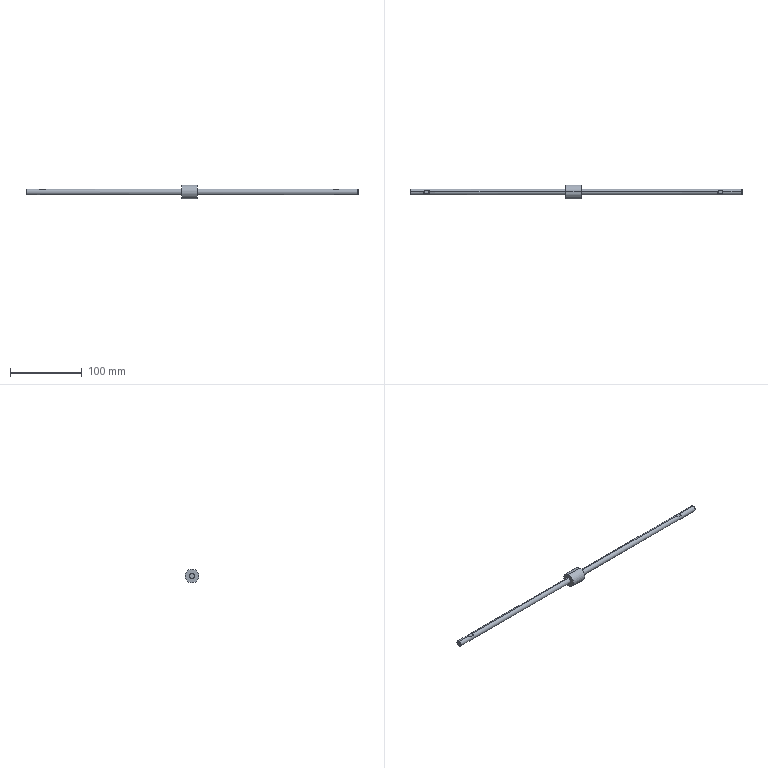Part | STEP file | _20MACJ15010Rod | 1 solid | 26 faces | box 463 x 19.5 x 19.5 mm | volume 28625 mm3 | plane 16 | cylinder 6 | cone 4 | commonest cylinder face diameters 8 x4 19.5 x2
STEP:
#1=CARTESIAN_POINT('',(462.233,0.,4.));
#2=VERTEX_POINT('',#1);
#3=CARTESIAN_POINT('',(462.233,0.,-4.));
#4=VERTEX_POINT('',#3);
#5=CARTESIAN_POINT('',(462.233,0.,0.));
#6=DIRECTION('',(-1.,0.,0.));
#7=DIRECTION('',(0.,0.,1.));
#8=AXIS2_PLACEMENT_3D('',#5,#6,#7);
#9=CIRCLE('',#8,4.);
#10=EDGE_CURVE('',#2,#4,#9,.T.);
#11=ORIENTED_EDGE('',*,*,#10,.T.);
#12=CARTESIAN_POINT('',(436.,0.,-4.));
#13=VERTEX_POINT('',#12);
#14=CARTESIAN_POINT('',(463.,0.,-4.));
#15=DIRECTION('',(-1.,0.,0.));
#16=VECTOR('',#15,1000.);
#17=LINE('',#14,#16);
#18=EDGE_CURVE('',#4,#13,#17,.T.);
#19=ORIENTED_EDGE('',*,*,#18,.T.);
#20=CARTESIAN_POINT('',(436.,2.646,-3.));
#21=VERTEX_POINT('',#20);
#22=CARTESIAN_POINT('',(436.,0.,0.));
#23=DIRECTION('',(1.,0.,0.));
#24=DIRECTION('',(0.,0.,1.));
#25=AXIS2_PLACEMENT_3D('',#22,#23,#24);
#26=CIRCLE('',#25,4.);
#27=EDGE_CURVE('',#13,#21,#26,.T.);
#28=ORIENTED_EDGE('',*,*,#27,.T.);
#29=CARTESIAN_POINT('',(430.,2.646,-3.));
#30=VERTEX_POINT('',#29);
#31=CARTESIAN_POINT('',(463.,2.646,-3.));
#32=DIRECTION('',(-1.,0.,0.));
#33=VECTOR('',#32,1000.);
#34=LINE('',#31,#33);
#35=EDGE_CURVE('',#21,#30,#34,.T.);
#36=ORIENTED_EDGE('',*,*,#35,.T.);
#37=CARTESIAN_POINT('',(429.,0.,-4.));
#38=VERTEX_POINT('',#37);
#39=CARTESIAN_POINT('',(430.,2.646,-3.));
#40=CARTESIAN_POINT('',(429.348,1.907,-3.652));
#41=CARTESIAN_POINT('',(429.,0.9852,-4.));
#42=CARTESIAN_POINT('',(429.,0.,-4.));
#43=(BOUNDED_CURVE()B_SPLINE_CURVE(3,(#39,#40,#41,#42),.UNSPECIFIED.,.F.,.T.)B_SPLINE_CURVE_WITH_KNOTS((4,4),(5.56,6.283),.UNSPECIFIED.)CURVE()GEOMETRIC_REPRESENTATION_ITEM()RATIONAL_B_SPLINE_CURVE((1.,0.9569,0.9569,1.))REPRESENTATION_ITEM(''));
#44=EDGE_CURVE('',#30,#38,#43,.T.);
#45=ORIENTED_EDGE('',*,*,#44,.T.);
#46=CARTESIAN_POINT('',(239.,0.,-4.));
#47=VERTEX_POINT('',#46);
#48=CARTESIAN_POINT('',(463.,0.,-4.));
#49=DIRECTION('',(-1.,0.,0.));
#50=VECTOR('',#49,1000.);
#51=LINE('',#48,#50);
#52=EDGE_CURVE('',#38,#47,#51,.T.);
#53=ORIENTED_EDGE('',*,*,#52,.T.);
#54=CARTESIAN_POINT('',(239.,0.,4.));
#55=VERTEX_POINT('',#54);
#56=CARTESIAN_POINT('',(239.,0.,0.));
#57=DIRECTION('',(1.,0.,0.));
#58=DIRECTION('',(0.,0.,1.));
#59=AXIS2_PLACEMENT_3D('',#56,#57,#58);
#60=CIRCLE('',#59,4.);
#61=EDGE_CURVE('',#47,#55,#60,.T.);
#62=ORIENTED_EDGE('',*,*,#61,.T.);
#63=CARTESIAN_POINT('',(429.,0.,4.));
#64=VERTEX_POINT('',#63);
#65=CARTESIAN_POINT('',(463.,0.,4.));
#66=DIRECTION('',(-1.,0.,0.));
#67=VECTOR('',#66,1000.);
#68=LINE('',#65,#67);
#69=EDGE_CURVE('',#64,#55,#68,.T.);
#70=ORIENTED_EDGE('',*,*,#69,.F.);
#71=CARTESIAN_POINT('',(430.,2.646,3.));
#72=VERTEX_POINT('',#71);
#73=CARTESIAN_POINT('',(429.,0.,4.));
#74=CARTESIAN_POINT('',(429.,0.9852,4.));
#75=CARTESIAN_POINT('',(429.348,1.907,3.652));
#76=CARTESIAN_POINT('',(430.,2.646,3.));
#77=(BOUNDED_CURVE()B_SPLINE_CURVE(3,(#73,#74,#75,#76),.UNSPECIFIED.,.F.,.T.)B_SPLINE_CURVE_WITH_KNOTS((4,4),(0.,0.7227),.UNSPECIFIED.)CURVE()GEOMETRIC_REPRESENTATION_ITEM()RATIONAL_B_SPLINE_CURVE((1.,0.9569,0.9569,1.))REPRESENTATION_ITEM(''));
#78=EDGE_CURVE('',#64,#72,#77,.T.);
#79=ORIENTED_EDGE('',*,*,#78,.T.);
#80=CARTESIAN_POINT('',(436.,2.646,3.));
#81=VERTEX_POINT('',#80);
#82=CARTESIAN_POINT('',(463.,2.646,3.));
#83=DIRECTION('',(1.,0.,0.));
#84=VECTOR('',#83,1000.);
#85=LINE('',#82,#84);
#86=EDGE_CURVE('',#72,#81,#85,.T.);
#87=ORIENTED_EDGE('',*,*,#86,.T.);
#88=CARTESIAN_POINT('',(436.,0.,4.));
#89=VERTEX_POINT('',#88);
#90=CARTESIAN_POINT('',(436.,0.,0.));
#91=DIRECTION('',(1.,0.,0.));
#92=DIRECTION('',(0.,0.,1.));
#93=AXIS2_PLACEMENT_3D('',#90,#91,#92);
#94=CIRCLE('',#93,4.);
#95=EDGE_CURVE('',#81,#89,#94,.T.);
#96=ORIENTED_EDGE('',*,*,#95,.T.);
#97=CARTESIAN_POINT('',(463.,0.,4.));
#98=DIRECTION('',(-1.,0.,0.));
#99=VECTOR('',#98,1000.);
#100=LINE('',#97,#99);
#101=EDGE_CURVE('',#2,#89,#100,.T.);
#102=ORIENTED_EDGE('',*,*,#101,.F.);
#103=EDGE_LOOP('',(#11,#19,#28,#36,#45,#53,#62,#70,#79,#87,#96,#102));
#104=FACE_OUTER_BOUND('',#103,.T.);
#105=CARTESIAN_POINT('',(463.,0.,0.));
#106=DIRECTION('',(-1.,0.,0.));
#107=DIRECTION('',(0.,0.,1.));
#108=AXIS2_PLACEMENT_3D('',#105,#106,#107);
#109=CYLINDRICAL_SURFACE('',#108,4.);
#110=ADVANCED_FACE('',(#104),#109,.T.);
#111=CARTESIAN_POINT('',(463.,0.,3.233));
#112=VERTEX_POINT('',#111);
#113=CARTESIAN_POINT('',(463.,0.,-3.233));
#114=VERTEX_POINT('',#113);
#115=CARTESIAN_POINT('',(463.,0.,0.));
#116=DIRECTION('',(-1.,0.,0.));
#117=DIRECTION('',(0.,0.,1.));
#118=AXIS2_PLACEMENT_3D('',#115,#116,#117);
#119=CIRCLE('',#118,3.233);
#120=EDGE_CURVE('',#112,#114,#119,.T.);
#121=ORIENTED_EDGE('',*,*,#120,.T.);
#122=CARTESIAN_POINT('',(462.233,0.,-4.));
#123=DIRECTION('',(-0.7071,0.,-0.7071));
#124=VECTOR('',#123,1000.);
#125=LINE('',#122,#124);
#126=EDGE_CURVE('',#114,#4,#125,.T.);
#127=ORIENTED_EDGE('',*,*,#126,.T.);
#128=ORIENTED_EDGE('',*,*,#10,.F.);
#129=CARTESIAN_POINT('',(462.233,0.,4.));
#130=DIRECTION('',(-0.7071,0.,0.7071));
#131=VECTOR('',#130,1000.);
#132=LINE('',#129,#131);
#133=EDGE_CURVE('',#112,#2,#132,.T.);
#134=ORIENTED_EDGE('',*,*,#133,.F.);
#135=EDGE_LOOP('',(#121,#127,#128,#134));
#136=FACE_OUTER_BOUND('',#135,.T.);
#137=CARTESIAN_POINT('',(462.233,0.,0.));
#138=DIRECTION('',(-1.,0.,0.));
#139=DIRECTION('',(0.,0.,1.));
#140=AXIS2_PLACEMENT_3D('',#137,#138,#139);
#141=CONICAL_SURFACE('',#140,4.,0.7854);
#142=ADVANCED_FACE('',(#136),#141,.T.);
#143=CARTESIAN_POINT('',(239.,0.,9.75));
#144=VERTEX_POINT('',#143);
#145=CARTESIAN_POINT('',(239.,0.,-9.75));
#146=VERTEX_POINT('',#145);
#147=CARTESIAN_POINT('',(239.,0.,0.));
#148=DIRECTION('',(-1.,0.,0.));
#149=DIRECTION('',(0.,0.,1.));
#150=AXIS2_PLACEMENT_3D('',#147,#148,#149);
#151=CIRCLE('',#150,9.75);
#152=EDGE_CURVE('',#144,#146,#151,.T.);
#153=ORIENTED_EDGE('',*,*,#152,.T.);
#154=CARTESIAN_POINT('',(217.,0.,-9.75));
#155=VERTEX_POINT('',#154);
#156=CARTESIAN_POINT('',(463.,0.,-9.75));
#157=DIRECTION('',(-1.,0.,0.));
#158=VECTOR('',#157,1000.);
#159=LINE('',#156,#158);
#160=EDGE_CURVE('',#146,#155,#159,.T.);
#161=ORIENTED_EDGE('',*,*,#160,.T.);
#162=CARTESIAN_POINT('',(217.,0.,9.75));
#163=VERTEX_POINT('',#162);
#164=CARTESIAN_POINT('',(217.,0.,0.));
#165=DIRECTION('',(1.,0.,0.));
#166=DIRECTION('',(0.,0.,1.));
#167=AXIS2_PLACEMENT_3D('',#164,#165,#166);
#168=CIRCLE('',#167,9.75);
#169=EDGE_CURVE('',#155,#163,#168,.T.);
#170=ORIENTED_EDGE('',*,*,#169,.T.);
#171=CARTESIAN_POINT('',(463.,0.,9.75));
#172=DIRECTION('',(-1.,0.,0.));
#173=VECTOR('',#172,1000.);
#174=LINE('',#171,#173);
#175=EDGE_CURVE('',#144,#163,#174,.T.);
#176=ORIENTED_EDGE('',*,*,#175,.F.);
#177=EDGE_LOOP('',(#153,#161,#170,#176));
#178=FACE_OUTER_BOUND('',#177,.T.);
#179=CARTESIAN_POINT('',(463.,0.,0.));
#180=DIRECTION('',(-1.,0.,0.));
#181=DIRECTION('',(0.,0.,1.));
#182=AXIS2_PLACEMENT_3D('',#179,#180,#181);
#183=CYLINDRICAL_SURFACE('',#182,9.75);
#184=ADVANCED_FACE('',(#178),#183,.T.);
#185=CARTESIAN_POINT('',(217.,0.,4.));
#186=VERTEX_POINT('',#185);
#187=CARTESIAN_POINT('',(217.,0.,-4.));
#188=VERTEX_POINT('',#187);
#189=CARTESIAN_POINT('',(217.,0.,0.));
#190=DIRECTION('',(-1.,0.,0.));
#191=DIRECTION('',(0.,0.,1.));
#192=AXIS2_PLACEMENT_3D('',#189,#190,#191);
#193=CIRCLE('',#192,4.);
#194=EDGE_CURVE('',#186,#188,#193,.T.);
#195=ORIENTED_EDGE('',*,*,#194,.T.);
#196=CARTESIAN_POINT('',(27.4,0.,-4.));
#197=VERTEX_POINT('',#196);
#198=CARTESIAN_POINT('',(463.,0.,-4.));
#199=DIRECTION('',(-1.,0.,0.));
#200=VECTOR('',#199,1000.);
#201=LINE('',#198,#200);
#202=EDGE_CURVE('',#188,#197,#201,.T.);
#203=ORIENTED_EDGE('',*,*,#202,.T.);
#204=CARTESIAN_POINT('',(26.4,2.646,-3.));
#205=VERTEX_POINT('',#204);
#206=CARTESIAN_POINT('',(27.4,0.,-4.));
#207=CARTESIAN_POINT('',(27.4,0.9852,-4.));
#208=CARTESIAN_POINT('',(27.052,1.907,-3.652));
#209=CARTESIAN_POINT('',(26.4,2.646,-3.));
#210=(BOUNDED_CURVE()B_SPLINE_CURVE(3,(#206,#207,#208,#209),.UNSPECIFIED.,.F.,.T.)B_SPLINE_CURVE_WITH_KNOTS((4,4),(3.142,3.864),.UNSPECIFIED.)CURVE()GEOMETRIC_REPRESENTATION_ITEM()RATIONAL_B_SPLINE_CURVE((1.,0.9569,0.9569,1.))REPRESENTATION_ITEM(''));
#211=EDGE_CURVE('',#197,#205,#210,.T.);
#212=ORIENTED_EDGE('',*,*,#211,.T.);
#213=CARTESIAN_POINT('',(20.,2.646,-3.));
#214=VERTEX_POINT('',#213);
#215=CARTESIAN_POINT('',(463.,2.646,-3.));
#216=DIRECTION('',(-1.,0.,0.));
#217=VECTOR('',#216,1000.);
#218=LINE('',#215,#217);
#219=EDGE_CURVE('',#205,#214,#218,.T.);
#220=ORIENTED_EDGE('',*,*,#219,.T.);
#221=CARTESIAN_POINT('',(19.,0.,-4.));
#222=VERTEX_POINT('',#221);
#223=CARTESIAN_POINT('',(20.,2.646,-3.));
#224=CARTESIAN_POINT('',(19.348,1.907,-3.652));
#225=CARTESIAN_POINT('',(19.,0.9852,-4.));
#226=CARTESIAN_POINT('',(19.,0.,-4.));
#227=(BOUNDED_CURVE()B_SPLINE_CURVE(3,(#223,#224,#225,#226),.UNSPECIFIED.,.F.,.T.)B_SPLINE_CURVE_WITH_KNOTS((4,4),(5.56,6.283),.UNSPECIFIED.)CURVE()GEOMETRIC_REPRESENTATION_ITEM()RATIONAL_B_SPLINE_CURVE((1.,0.9569,0.9569,1.))REPRESENTATION_ITEM(''));
#228=EDGE_CURVE('',#214,#222,#227,.T.);
#229=ORIENTED_EDGE('',*,*,#228,.T.);
#230=CARTESIAN_POINT('',(0.767,0.,-4.));
#231=VERTEX_POINT('',#230);
#232=CARTESIAN_POINT('',(463.,0.,-4.));
#233=DIRECTION('',(-1.,0.,0.));
#234=VECTOR('',#233,1000.);
#235=LINE('',#232,#234);
#236=EDGE_CURVE('',#222,#231,#235,.T.);
#237=ORIENTED_EDGE('',*,*,#236,.T.);
#238=CARTESIAN_POINT('',(0.767,4.,0.));
#239=VERTEX_POINT('',#238);
#240=CARTESIAN_POINT('',(0.767,0.,0.));
#241=DIRECTION('',(1.,0.,0.));
#242=DIRECTION('',(0.,0.,1.));
#243=AXIS2_PLACEMENT_3D('',#240,#241,#242);
#244=CIRCLE('',#243,4.);
#245=EDGE_CURVE('',#231,#239,#244,.T.);
#246=ORIENTED_EDGE('',*,*,#245,.T.);
#247=CARTESIAN_POINT('',(0.767,0.,4.));
#248=VERTEX_POINT('',#247);
#249=CARTESIAN_POINT('',(0.767,0.,0.));
#250=DIRECTION('',(1.,0.,0.));
#251=DIRECTION('',(0.,0.,1.));
#252=AXIS2_PLACEMENT_3D('',#249,#250,#251);
#253=CIRCLE('',#252,4.);
#254=EDGE_CURVE('',#239,#248,#253,.T.);
#255=ORIENTED_EDGE('',*,*,#254,.T.);
#256=CARTESIAN_POINT('',(19.,0.,4.));
#257=VERTEX_POINT('',#256);
#258=CARTESIAN_POINT('',(463.,0.,4.));
#259=DIRECTION('',(-1.,0.,0.));
#260=VECTOR('',#259,1000.);
#261=LINE('',#258,#260);
#262=EDGE_CURVE('',#257,#248,#261,.T.);
#263=ORIENTED_EDGE('',*,*,#262,.F.);
#264=CARTESIAN_POINT('',(20.,2.646,3.));
#265=VERTEX_POINT('',#264);
#266=CARTESIAN_POINT('',(19.,0.,4.));
#267=CARTESIAN_POINT('',(19.,0.9852,4.));
#268=CARTESIAN_POINT('',(19.348,1.907,3.652));
#269=CARTESIAN_POINT('',(20.,2.646,3.));
#270=(BOUNDED_CURVE()B_SPLINE_CURVE(3,(#266,#267,#268,#269),.UNSPECIFIED.,.F.,.F.)B_SPLINE_CURVE_WITH_KNOTS((4,4),(0.,0.7227),.UNSPECIFIED.)CURVE()GEOMETRIC_REPRESENTATION_ITEM()RATIONAL_B_SPLINE_CURVE((1.,0.9569,0.9569,1.))REPRESENTATION_ITEM(''));
#271=EDGE_CURVE('',#257,#265,#270,.T.);
#272=ORIENTED_EDGE('',*,*,#271,.T.);
#273=CARTESIAN_POINT('',(26.4,2.646,3.));
#274=VERTEX_POINT('',#273);
#275=CARTESIAN_POINT('',(463.,2.646,3.));
#276=DIRECTION('',(1.,0.,0.));
#277=VECTOR('',#276,1000.);
#278=LINE('',#275,#277);
#279=EDGE_CURVE('',#265,#274,#278,.T.);
#280=ORIENTED_EDGE('',*,*,#279,.T.);
#281=CARTESIAN_POINT('',(27.4,0.,4.));
#282=VERTEX_POINT('',#281);
#283=CARTESIAN_POINT('',(26.4,2.646,3.));
#284=CARTESIAN_POINT('',(27.052,1.907,3.652));
#285=CARTESIAN_POINT('',(27.4,0.9852,4.));
#286=CARTESIAN_POINT('',(27.4,0.,4.));
#287=(BOUNDED_CURVE()B_SPLINE_CURVE(3,(#283,#284,#285,#286),.UNSPECIFIED.,.F.,.F.)B_SPLINE_CURVE_WITH_KNOTS((4,4),(2.419,3.142),.UNSPECIFIED.)CURVE()GEOMETRIC_REPRESENTATION_ITEM()RATIONAL_B_SPLINE_CURVE((1.,0.9569,0.9569,1.))REPRESENTATION_ITEM(''));
#288=EDGE_CURVE('',#274,#282,#287,.T.);
#289=ORIENTED_EDGE('',*,*,#288,.T.);
#290=CARTESIAN_POINT('',(463.,0.,4.));
#291=DIRECTION('',(-1.,0.,0.));
#292=VECTOR('',#291,1000.);
#293=LINE('',#290,#292);
#294=EDGE_CURVE('',#186,#282,#293,.T.);
#295=ORIENTED_EDGE('',*,*,#294,.F.);
#296=EDGE_LOOP('',(#195,#203,#212,#220,#229,#237,#246,#255,#263,#272,#280,#289,#295));
#297=FACE_OUTER_BOUND('',#296,.T.);
#298=CARTESIAN_POINT('',(463.,0.,0.));
#299=DIRECTION('',(-1.,0.,0.));
#300=DIRECTION('',(0.,0.,1.));
#301=AXIS2_PLACEMENT_3D('',#298,#299,#300);
#302=CYLINDRICAL_SURFACE('',#301,4.);
#303=ADVANCED_FACE('',(#297),#302,.T.);
#304=CARTESIAN_POINT('',(0.,3.233,0.));
#305=VERTEX_POINT('',#304);
#306=CARTESIAN_POINT('',(0.,-3.233,0.));
#307=VERTEX_POINT('',#306);
#308=CARTESIAN_POINT('',(0.,0.,0.));
#309=DIRECTION('',(1.,0.,0.));
#310=DIRECTION('',(0.,1.,0.));
#311=AXIS2_PLACEMENT_3D('',#308,#309,#310);
#312=CIRCLE('',#311,3.233);
#313=EDGE_CURVE('',#305,#307,#312,.T.);
#314=ORIENTED_EDGE('',*,*,#313,.T.);
#315=CARTESIAN_POINT('',(0.767,-4.,0.));
#316=VERTEX_POINT('',#315);
#317=CARTESIAN_POINT('',(0.767,-4.,0.));
#318=DIRECTION('',(0.7071,-0.7071,0.));
#319=VECTOR('',#318,1000.);
#320=LINE('',#317,#319);
#321=EDGE_CURVE('',#307,#316,#320,.T.);
#322=ORIENTED_EDGE('',*,*,#321,.T.);
#323=CARTESIAN_POINT('',(0.767,0.,0.));
#324=DIRECTION('',(1.,0.,0.));
#325=DIRECTION('',(0.,0.,1.));
#326=AXIS2_PLACEMENT_3D('',#323,#324,#325);
#327=CIRCLE('',#326,4.);
#328=EDGE_CURVE('',#248,#316,#327,.T.);
#329=ORIENTED_EDGE('',*,*,#328,.F.);
#330=ORIENTED_EDGE('',*,*,#254,.F.);
#331=CARTESIAN_POINT('',(0.767,4.,0.));
#332=DIRECTION('',(0.7071,0.7071,0.));
#333=VECTOR('',#332,1000.);
#334=LINE('',#331,#333);
#335=EDGE_CURVE('',#305,#239,#334,.T.);
#336=ORIENTED_EDGE('',*,*,#335,.F.);
#337=EDGE_LOOP('',(#314,#322,#329,#330,#336));
#338=FACE_OUTER_BOUND('',#337,.T.);
#339=CARTESIAN_POINT('',(0.767,0.,0.));
#340=DIRECTION('',(1.,0.,0.));
#341=DIRECTION('',(0.,1.,0.));
#342=AXIS2_PLACEMENT_3D('',#339,#340,#341);
#343=CONICAL_SURFACE('',#342,4.,0.7854);
#344=ADVANCED_FACE('',(#338),#343,.T.);
#345=ORIENTED_EDGE('',*,*,#18,.F.);
#346=CARTESIAN_POINT('',(462.233,0.,0.));
#347=DIRECTION('',(-1.,0.,0.));
#348=DIRECTION('',(0.,0.,1.));
#349=AXIS2_PLACEMENT_3D('',#346,#347,#348);
#350=CIRCLE('',#349,4.);
#351=EDGE_CURVE('',#4,#2,#350,.T.);
#352=ORIENTED_EDGE('',*,*,#351,.T.);
#353=ORIENTED_EDGE('',*,*,#101,.T.);
#354=CARTESIAN_POINT('',(436.,-2.646,3.));
#355=VERTEX_POINT('',#354);
#356=CARTESIAN_POINT('',(436.,0.,0.));
#357=DIRECTION('',(1.,0.,0.));
#358=DIRECTION('',(0.,0.,1.));
#359=AXIS2_PLACEMENT_3D('',#356,#357,#358);
#360=CIRCLE('',#359,4.);
#361=EDGE_CURVE('',#89,#355,#360,.T.);
#362=ORIENTED_EDGE('',*,*,#361,.T.);
#363=CARTESIAN_POINT('',(430.,-2.646,3.));
#364=VERTEX_POINT('',#363);
#365=CARTESIAN_POINT('',(463.,-2.646,3.));
#366=DIRECTION('',(-1.,0.,0.));
#367=VECTOR('',#366,1000.);
#368=LINE('',#365,#367);
#369=EDGE_CURVE('',#355,#364,#368,.T.);
#370=ORIENTED_EDGE('',*,*,#369,.T.);
#371=CARTESIAN_POINT('',(430.,-2.646,3.));
#372=CARTESIAN_POINT('',(429.348,-1.907,3.652));
#373=CARTESIAN_POINT('',(429.,-0.9852,4.));
#374=CARTESIAN_POINT('',(429.,0.,4.));
#375=(BOUNDED_CURVE()B_SPLINE_CURVE(3,(#371,#372,#373,#374),.UNSPECIFIED.,.F.,.F.)B_SPLINE_CURVE_WITH_KNOTS((4,4),(5.56,6.283),.UNSPECIFIED.)CURVE()GEOMETRIC_REPRESENTATION_ITEM()RATIONAL_B_SPLINE_CURVE((1.,0.9569,0.9569,1.))REPRESENTATION_ITEM(''));
#376=EDGE_CURVE('',#364,#64,#375,.T.);
#377=ORIENTED_EDGE('',*,*,#376,.T.);
#378=ORIENTED_EDGE('',*,*,#69,.T.);
#379=CARTESIAN_POINT('',(239.,0.,0.));
#380=DIRECTION('',(1.,0.,0.));
#381=DIRECTION('',(0.,0.,1.));
#382=AXIS2_PLACEMENT_3D('',#379,#380,#381);
#383=CIRCLE('',#382,4.);
#384=EDGE_CURVE('',#55,#47,#383,.T.);
#385=ORIENTED_EDGE('',*,*,#384,.T.);
#386=ORIENTED_EDGE('',*,*,#52,.F.);
#387=CARTESIAN_POINT('',(430.,-2.646,-3.));
#388=VERTEX_POINT('',#387);
#389=CARTESIAN_POINT('',(429.,0.,-4.));
#390=CARTESIAN_POINT('',(429.,-0.9852,-4.));
#391=CARTESIAN_POINT('',(429.348,-1.907,-3.652));
#392=CARTESIAN_POINT('',(430.,-2.646,-3.));
#393=(BOUNDED_CURVE()B_SPLINE_CURVE(3,(#389,#390,#391,#392),.UNSPECIFIED.,.F.,.F.)B_SPLINE_CURVE_WITH_KNOTS((4,4),(0.,0.7227),.UNSPECIFIED.)CURVE()GEOMETRIC_REPRESENTATION_ITEM()RATIONAL_B_SPLINE_CURVE((1.,0.9569,0.9569,1.))REPRESENTATION_ITEM(''));
#394=EDGE_CURVE('',#38,#388,#393,.T.);
#395=ORIENTED_EDGE('',*,*,#394,.T.);
#396=CARTESIAN_POINT('',(436.,-2.646,-3.));
#397=VERTEX_POINT('',#396);
#398=CARTESIAN_POINT('',(463.,-2.646,-3.));
#399=DIRECTION('',(1.,0.,0.));
#400=VECTOR('',#399,1000.);
#401=LINE('',#398,#400);
#402=EDGE_CURVE('',#388,#397,#401,.T.);
#403=ORIENTED_EDGE('',*,*,#402,.T.);
#404=CARTESIAN_POINT('',(436.,0.,0.));
#405=DIRECTION('',(1.,0.,0.));
#406=DIRECTION('',(0.,0.,1.));
#407=AXIS2_PLACEMENT_3D('',#404,#405,#406);
#408=CIRCLE('',#407,4.);
#409=EDGE_CURVE('',#397,#13,#408,.T.);
#410=ORIENTED_EDGE('',*,*,#409,.T.);
#411=EDGE_LOOP('',(#345,#352,#353,#362,#370,#377,#378,#385,#386,#395,#403,#410));
#412=FACE_OUTER_BOUND('',#411,.T.);
#413=CARTESIAN_POINT('',(463.,0.,0.));
#414=DIRECTION('',(-1.,0.,0.));
#415=DIRECTION('',(0.,0.,1.));
#416=AXIS2_PLACEMENT_3D('',#413,#414,#415);
#417=CYLINDRICAL_SURFACE('',#416,4.);
#418=ADVANCED_FACE('',(#412),#417,.T.);
#419=ORIENTED_EDGE('',*,*,#402,.F.);
#420=CARTESIAN_POINT('',(430.,3.,-3.));
#421=DIRECTION('',(0.,1.,0.));
#422=VECTOR('',#421,1000.);
#423=LINE('',#420,#422);
#424=EDGE_CURVE('',#388,#30,#423,.T.);
#425=ORIENTED_EDGE('',*,*,#424,.T.);
#426=ORIENTED_EDGE('',*,*,#35,.F.);
#427=CARTESIAN_POINT('',(436.,3.,-3.));
#428=DIRECTION('',(0.,-1.,0.));
#429=VECTOR('',#428,1000.);
#430=LINE('',#427,#429);
#431=EDGE_CURVE('',#21,#397,#430,.T.);
#432=ORIENTED_EDGE('',*,*,#431,.T.);
#433=EDGE_LOOP('',(#419,#425,#426,#432));
#434=FACE_OUTER_BOUND('',#433,.T.);
#435=CARTESIAN_POINT('',(430.,3.,-3.));
#436=DIRECTION('',(0.,0.,-1.));
#437=DIRECTION('',(-1.,0.,0.));
#438=AXIS2_PLACEMENT_3D('',#435,#436,#437);
#439=PLANE('',#438);
#440=ADVANCED_FACE('',(#434),#439,.T.);
#441=ORIENTED_EDGE('',*,*,#409,.F.);
#442=ORIENTED_EDGE('',*,*,#431,.F.);
#443=ORIENTED_EDGE('',*,*,#27,.F.);
#444=EDGE_LOOP('',(#441,#442,#443));
#445=FACE_OUTER_BOUND('',#444,.T.);
#446=CARTESIAN_POINT('',(436.,3.,-3.));
#447=DIRECTION('',(-1.,0.,0.));
#448=DIRECTION('',(0.,0.,1.));
#449=AXIS2_PLACEMENT_3D('',#446,#447,#448);
#450=PLANE('',#449);
#451=ADVANCED_FACE('',(#445),#450,.T.);
#452=ORIENTED_EDGE('',*,*,#44,.F.);
#453=ORIENTED_EDGE('',*,*,#424,.F.);
#454=ORIENTED_EDGE('',*,*,#394,.F.);
#455=EDGE_LOOP('',(#452,#453,#454));
#456=FACE_OUTER_BOUND('',#455,.T.);
#457=CARTESIAN_POINT('',(421.,3.,-12.));
#458=DIRECTION('',(0.7071,0.,-0.7071));
#459=DIRECTION('',(-0.7071,0.,-0.7071));
#460=AXIS2_PLACEMENT_3D('',#457,#458,#459);
#461=PLANE('',#460);
#462=ADVANCED_FACE('',(#456),#461,.T.);
#463=ORIENTED_EDGE('',*,*,#152,.F.);
#464=CARTESIAN_POINT('',(239.,0.,0.));
#465=DIRECTION('',(-1.,0.,0.));
#466=DIRECTION('',(0.,0.,1.));
#467=AXIS2_PLACEMENT_3D('',#464,#465,#466);
#468=CIRCLE('',#467,9.75);
#469=EDGE_CURVE('',#146,#144,#468,.T.);
#470=ORIENTED_EDGE('',*,*,#469,.F.);
#471=EDGE_LOOP('',(#463,#470));
#472=FACE_OUTER_BOUND('',#471,.T.);
#473=ORIENTED_EDGE('',*,*,#384,.F.);
#474=ORIENTED_EDGE('',*,*,#61,.F.);
#475=EDGE_LOOP('',(#473,#474));
#476=FACE_BOUND('',#475,.T.);
#477=CARTESIAN_POINT('',(239.,9.75,0.));
#478=DIRECTION('',(-1.,0.,0.));
#479=DIRECTION('',(0.,0.,1.));
#480=AXIS2_PLACEMENT_3D('',#477,#478,#479);
#481=PLANE('',#480);
#482=ADVANCED_FACE('',(#472,#476),#481,.F.);
#483=ORIENTED_EDGE('',*,*,#95,.F.);
#484=CARTESIAN_POINT('',(436.,3.,3.));
#485=DIRECTION('',(0.,-1.,0.));
#486=VECTOR('',#485,1000.);
#487=LINE('',#484,#486);
#488=EDGE_CURVE('',#81,#355,#487,.T.);
#489=ORIENTED_EDGE('',*,*,#488,.T.);
#490=ORIENTED_EDGE('',*,*,#361,.F.);
#491=EDGE_LOOP('',(#483,#489,#490));
#492=FACE_OUTER_BOUND('',#491,.T.);
#493=CARTESIAN_POINT('',(436.,3.,10.));
#494=DIRECTION('',(-1.,0.,0.));
#495=DIRECTION('',(0.,0.,1.));
#496=AXIS2_PLACEMENT_3D('',#493,#494,#495);
#497=PLANE('',#496);
#498=ADVANCED_FACE('',(#492),#497,.T.);
#499=ORIENTED_EDGE('',*,*,#86,.F.);
#500=CARTESIAN_POINT('',(430.,3.,3.));
#501=DIRECTION('',(0.,-1.,0.));
#502=VECTOR('',#501,1000.);
#503=LINE('',#500,#502);
#504=EDGE_CURVE('',#72,#364,#503,.T.);
#505=ORIENTED_EDGE('',*,*,#504,.T.);
#506=ORIENTED_EDGE('',*,*,#369,.F.);
#507=ORIENTED_EDGE('',*,*,#488,.F.);
#508=EDGE_LOOP('',(#499,#505,#506,#507));
#509=FACE_OUTER_BOUND('',#508,.T.);
#510=CARTESIAN_POINT('',(436.,3.,3.));
#511=DIRECTION('',(0.,0.,1.));
#512=DIRECTION('',(1.,0.,0.));
#513=AXIS2_PLACEMENT_3D('',#510,#511,#512);
#514=PLANE('',#513);
#515=ADVANCED_FACE('',(#509),#514,.T.);
#516=ORIENTED_EDGE('',*,*,#376,.F.);
#517=ORIENTED_EDGE('',*,*,#504,.F.);
#518=ORIENTED_EDGE('',*,*,#78,.F.);
#519=EDGE_LOOP('',(#516,#517,#518));
#520=FACE_OUTER_BOUND('',#519,.T.);
#521=CARTESIAN_POINT('',(430.,3.,3.));
#522=DIRECTION('',(0.7071,0.,0.7071));
#523=DIRECTION('',(0.7071,0.,-0.7071));
#524=AXIS2_PLACEMENT_3D('',#521,#522,#523);
#525=PLANE('',#524);
#526=ADVANCED_FACE('',(#520),#525,.T.);
#527=ORIENTED_EDGE('',*,*,#126,.F.);
#528=CARTESIAN_POINT('',(463.,0.,0.));
#529=DIRECTION('',(-1.,0.,0.));
#530=DIRECTION('',(0.,0.,1.));
#531=AXIS2_PLACEMENT_3D('',#528,#529,#530);
#532=CIRCLE('',#531,3.233);
#533=EDGE_CURVE('',#114,#112,#532,.T.);
#534=ORIENTED_EDGE('',*,*,#533,.T.);
#535=ORIENTED_EDGE('',*,*,#133,.T.);
#536=ORIENTED_EDGE('',*,*,#351,.F.);
#537=EDGE_LOOP('',(#527,#534,#535,#536));
#538=FACE_OUTER_BOUND('',#537,.T.);
#539=CARTESIAN_POINT('',(462.233,0.,0.));
#540=DIRECTION('',(-1.,0.,0.));
#541=DIRECTION('',(0.,0.,1.));
#542=AXIS2_PLACEMENT_3D('',#539,#540,#541);
#543=CONICAL_SURFACE('',#542,4.,0.7854);
#544=ADVANCED_FACE('',(#538),#543,.T.);
#545=ORIENTED_EDGE('',*,*,#160,.F.);
#546=ORIENTED_EDGE('',*,*,#469,.T.);
#547=ORIENTED_EDGE('',*,*,#175,.T.);
#548=CARTESIAN_POINT('',(217.,0.,0.));
#549=DIRECTION('',(1.,0.,0.));
#550=DIRECTION('',(0.,0.,1.));
#551=AXIS2_PLACEMENT_3D('',#548,#549,#550);
#552=CIRCLE('',#551,9.75);
#553=EDGE_CURVE('',#163,#155,#552,.T.);
#554=ORIENTED_EDGE('',*,*,#553,.T.);
#555=EDGE_LOOP('',(#545,#546,#547,#554));
#556=FACE_OUTER_BOUND('',#555,.T.);
#557=CARTESIAN_POINT('',(463.,0.,0.));
#558=DIRECTION('',(-1.,0.,0.));
#559=DIRECTION('',(0.,0.,1.));
#560=AXIS2_PLACEMENT_3D('',#557,#558,#559);
#561=CYLINDRICAL_SURFACE('',#560,9.75);
#562=ADVANCED_FACE('',(#556),#561,.T.);
#563=ORIENTED_EDGE('',*,*,#120,.F.);
#564=ORIENTED_EDGE('',*,*,#533,.F.);
#565=EDGE_LOOP('',(#563,#564));
#566=FACE_OUTER_BOUND('',#565,.T.);
#567=CARTESIAN_POINT('',(463.,3.233,0.));
#568=DIRECTION('',(-1.,0.,0.));
#569=DIRECTION('',(0.,0.,1.));
#570=AXIS2_PLACEMENT_3D('',#567,#568,#569);
#571=PLANE('',#570);
#572=ADVANCED_FACE('',(#566),#571,.F.);
#573=ORIENTED_EDGE('',*,*,#194,.F.);
#574=CARTESIAN_POINT('',(217.,0.,0.));
#575=DIRECTION('',(-1.,0.,0.));
#576=DIRECTION('',(0.,0.,1.));
#577=AXIS2_PLACEMENT_3D('',#574,#575,#576);
#578=CIRCLE('',#577,4.);
#579=EDGE_CURVE('',#188,#186,#578,.T.);
#580=ORIENTED_EDGE('',*,*,#579,.F.);
#581=EDGE_LOOP('',(#573,#580));
#582=FACE_BOUND('',#581,.T.);
#583=ORIENTED_EDGE('',*,*,#553,.F.);
#584=ORIENTED_EDGE('',*,*,#169,.F.);
#585=EDGE_LOOP('',(#583,#584));
#586=FACE_OUTER_BOUND('',#585,.T.);
#587=CARTESIAN_POINT('',(217.,4.,0.));
#588=DIRECTION('',(1.,0.,0.));
#589=DIRECTION('',(0.,0.,-1.));
#590=AXIS2_PLACEMENT_3D('',#587,#588,#589);
#591=PLANE('',#590);
#592=ADVANCED_FACE('',(#582,#586),#591,.F.);
#593=ORIENTED_EDGE('',*,*,#202,.F.);
#594=ORIENTED_EDGE('',*,*,#579,.T.);
#595=ORIENTED_EDGE('',*,*,#294,.T.);
#596=CARTESIAN_POINT('',(26.4,-2.646,3.));
#597=VERTEX_POINT('',#596);
#598=CARTESIAN_POINT('',(27.4,0.,4.));
#599=CARTESIAN_POINT('',(27.4,-0.9852,4.));
#600=CARTESIAN_POINT('',(27.052,-1.907,3.652));
#601=CARTESIAN_POINT('',(26.4,-2.646,3.));
#602=(BOUNDED_CURVE()B_SPLINE_CURVE(3,(#598,#599,#600,#601),.UNSPECIFIED.,.F.,.F.)B_SPLINE_CURVE_WITH_KNOTS((4,4),(3.142,3.864),.UNSPECIFIED.)CURVE()GEOMETRIC_REPRESENTATION_ITEM()RATIONAL_B_SPLINE_CURVE((1.,0.9569,0.9569,1.))REPRESENTATION_ITEM(''));
#603=EDGE_CURVE('',#282,#597,#602,.T.);
#604=ORIENTED_EDGE('',*,*,#603,.T.);
#605=CARTESIAN_POINT('',(20.,-2.646,3.));
#606=VERTEX_POINT('',#605);
#607=CARTESIAN_POINT('',(463.,-2.646,3.));
#608=DIRECTION('',(-1.,0.,0.));
#609=VECTOR('',#608,1000.);
#610=LINE('',#607,#609);
#611=EDGE_CURVE('',#597,#606,#610,.T.);
#612=ORIENTED_EDGE('',*,*,#611,.T.);
#613=CARTESIAN_POINT('',(20.,-2.646,3.));
#614=CARTESIAN_POINT('',(19.348,-1.907,3.652));
#615=CARTESIAN_POINT('',(19.,-0.9852,4.));
#616=CARTESIAN_POINT('',(19.,0.,4.));
#617=(BOUNDED_CURVE()B_SPLINE_CURVE(3,(#613,#614,#615,#616),.UNSPECIFIED.,.F.,.F.)B_SPLINE_CURVE_WITH_KNOTS((4,4),(5.56,6.283),.UNSPECIFIED.)CURVE()GEOMETRIC_REPRESENTATION_ITEM()RATIONAL_B_SPLINE_CURVE((1.,0.9569,0.9569,1.))REPRESENTATION_ITEM(''));
#618=EDGE_CURVE('',#606,#257,#617,.T.);
#619=ORIENTED_EDGE('',*,*,#618,.T.);
#620=ORIENTED_EDGE('',*,*,#262,.T.);
#621=ORIENTED_EDGE('',*,*,#328,.T.);
#622=CARTESIAN_POINT('',(0.767,0.,0.));
#623=DIRECTION('',(1.,0.,0.));
#624=DIRECTION('',(0.,0.,1.));
#625=AXIS2_PLACEMENT_3D('',#622,#623,#624);
#626=CIRCLE('',#625,4.);
#627=EDGE_CURVE('',#316,#231,#626,.T.);
#628=ORIENTED_EDGE('',*,*,#627,.T.);
#629=ORIENTED_EDGE('',*,*,#236,.F.);
#630=CARTESIAN_POINT('',(20.,-2.646,-3.));
#631=VERTEX_POINT('',#630);
#632=CARTESIAN_POINT('',(19.,0.,-4.));
#633=CARTESIAN_POINT('',(19.,-0.9852,-4.));
#634=CARTESIAN_POINT('',(19.348,-1.907,-3.652));
#635=CARTESIAN_POINT('',(20.,-2.646,-3.));
#636=(BOUNDED_CURVE()B_SPLINE_CURVE(3,(#632,#633,#634,#635),.UNSPECIFIED.,.F.,.F.)B_SPLINE_CURVE_WITH_KNOTS((4,4),(0.,0.7227),.UNSPECIFIED.)CURVE()GEOMETRIC_REPRESENTATION_ITEM()RATIONAL_B_SPLINE_CURVE((1.,0.9569,0.9569,1.))REPRESENTATION_ITEM(''));
#637=EDGE_CURVE('',#222,#631,#636,.T.);
#638=ORIENTED_EDGE('',*,*,#637,.T.);
#639=CARTESIAN_POINT('',(26.4,-2.646,-3.));
#640=VERTEX_POINT('',#639);
#641=CARTESIAN_POINT('',(463.,-2.646,-3.));
#642=DIRECTION('',(1.,0.,0.));
#643=VECTOR('',#642,1000.);
#644=LINE('',#641,#643);
#645=EDGE_CURVE('',#631,#640,#644,.T.);
#646=ORIENTED_EDGE('',*,*,#645,.T.);
#647=CARTESIAN_POINT('',(26.4,-2.646,-3.));
#648=CARTESIAN_POINT('',(27.052,-1.907,-3.652));
#649=CARTESIAN_POINT('',(27.4,-0.9852,-4.));
#650=CARTESIAN_POINT('',(27.4,0.,-4.));
#651=(BOUNDED_CURVE()B_SPLINE_CURVE(3,(#647,#648,#649,#650),.UNSPECIFIED.,.F.,.F.)B_SPLINE_CURVE_WITH_KNOTS((4,4),(2.419,3.142),.UNSPECIFIED.)CURVE()GEOMETRIC_REPRESENTATION_ITEM()RATIONAL_B_SPLINE_CURVE((1.,0.9569,0.9569,1.))REPRESENTATION_ITEM(''));
#652=EDGE_CURVE('',#640,#197,#651,.T.);
#653=ORIENTED_EDGE('',*,*,#652,.T.);
#654=EDGE_LOOP('',(#593,#594,#595,#604,#612,#619,#620,#621,#628,#629,#638,#646,#653));
#655=FACE_OUTER_BOUND('',#654,.T.);
#656=CARTESIAN_POINT('',(463.,0.,0.));
#657=DIRECTION('',(-1.,0.,0.));
#658=DIRECTION('',(0.,0.,1.));
#659=AXIS2_PLACEMENT_3D('',#656,#657,#658);
#660=CYLINDRICAL_SURFACE('',#659,4.);
#661=ADVANCED_FACE('',(#655),#660,.T.);
#662=ORIENTED_EDGE('',*,*,#279,.F.);
#663=CARTESIAN_POINT('',(20.,3.,3.));
#664=DIRECTION('',(0.,-1.,0.));
#665=VECTOR('',#664,1000.);
#666=LINE('',#663,#665);
#667=EDGE_CURVE('',#265,#606,#666,.T.);
#668=ORIENTED_EDGE('',*,*,#667,.T.);
#669=ORIENTED_EDGE('',*,*,#611,.F.);
#670=CARTESIAN_POINT('',(26.4,3.,3.));
#671=DIRECTION('',(0.,1.,0.));
#672=VECTOR('',#671,1000.);
#673=LINE('',#670,#672);
#674=EDGE_CURVE('',#597,#274,#673,.T.);
#675=ORIENTED_EDGE('',*,*,#674,.T.);
#676=EDGE_LOOP('',(#662,#668,#669,#675));
#677=FACE_OUTER_BOUND('',#676,.T.);
#678=CARTESIAN_POINT('',(26.4,3.,3.));
#679=DIRECTION('',(0.,0.,1.));
#680=DIRECTION('',(1.,0.,0.));
#681=AXIS2_PLACEMENT_3D('',#678,#679,#680);
#682=PLANE('',#681);
#683=ADVANCED_FACE('',(#677),#682,.T.);
#684=ORIENTED_EDGE('',*,*,#618,.F.);
#685=ORIENTED_EDGE('',*,*,#667,.F.);
#686=ORIENTED_EDGE('',*,*,#271,.F.);
#687=EDGE_LOOP('',(#684,#685,#686));
#688=FACE_OUTER_BOUND('',#687,.T.);
#689=CARTESIAN_POINT('',(20.,3.,3.));
#690=DIRECTION('',(0.7071,0.,0.7071));
#691=DIRECTION('',(0.7071,0.,-0.7071));
#692=AXIS2_PLACEMENT_3D('',#689,#690,#691);
#693=PLANE('',#692);
#694=ADVANCED_FACE('',(#688),#693,.T.);
#695=ORIENTED_EDGE('',*,*,#288,.F.);
#696=ORIENTED_EDGE('',*,*,#674,.F.);
#697=ORIENTED_EDGE('',*,*,#603,.F.);
#698=EDGE_LOOP('',(#695,#696,#697));
#699=FACE_OUTER_BOUND('',#698,.T.);
#700=CARTESIAN_POINT('',(35.4,3.,12.));
#701=DIRECTION('',(-0.7071,0.,0.7071));
#702=DIRECTION('',(0.7071,0.,0.7071));
#703=AXIS2_PLACEMENT_3D('',#700,#701,#702);
#704=PLANE('',#703);
#705=ADVANCED_FACE('',(#699),#704,.T.);
#706=ORIENTED_EDGE('',*,*,#321,.F.);
#707=CARTESIAN_POINT('',(0.,0.,0.));
#708=DIRECTION('',(1.,0.,0.));
#709=DIRECTION('',(0.,1.,0.));
#710=AXIS2_PLACEMENT_3D('',#707,#708,#709);
#711=CIRCLE('',#710,3.233);
#712=EDGE_CURVE('',#307,#305,#711,.T.);
#713=ORIENTED_EDGE('',*,*,#712,.T.);
#714=ORIENTED_EDGE('',*,*,#335,.T.);
#715=ORIENTED_EDGE('',*,*,#245,.F.);
#716=ORIENTED_EDGE('',*,*,#627,.F.);
#717=EDGE_LOOP('',(#706,#713,#714,#715,#716));
#718=FACE_OUTER_BOUND('',#717,.T.);
#719=CARTESIAN_POINT('',(0.767,0.,0.));
#720=DIRECTION('',(1.,0.,0.));
#721=DIRECTION('',(0.,1.,0.));
#722=AXIS2_PLACEMENT_3D('',#719,#720,#721);
#723=CONICAL_SURFACE('',#722,4.,0.7854);
#724=ADVANCED_FACE('',(#718),#723,.T.);
#725=ORIENTED_EDGE('',*,*,#645,.F.);
#726=CARTESIAN_POINT('',(20.,3.,-3.));
#727=DIRECTION('',(0.,1.,0.));
#728=VECTOR('',#727,1000.);
#729=LINE('',#726,#728);
#730=EDGE_CURVE('',#631,#214,#729,.T.);
#731=ORIENTED_EDGE('',*,*,#730,.T.);
#732=ORIENTED_EDGE('',*,*,#219,.F.);
#733=CARTESIAN_POINT('',(26.4,3.,-3.));
#734=DIRECTION('',(0.,-1.,0.));
#735=VECTOR('',#734,1000.);
#736=LINE('',#733,#735);
#737=EDGE_CURVE('',#205,#640,#736,.T.);
#738=ORIENTED_EDGE('',*,*,#737,.T.);
#739=EDGE_LOOP('',(#725,#731,#732,#738));
#740=FACE_OUTER_BOUND('',#739,.T.);
#741=CARTESIAN_POINT('',(20.,3.,-3.));
#742=DIRECTION('',(0.,0.,-1.));
#743=DIRECTION('',(-1.,0.,0.));
#744=AXIS2_PLACEMENT_3D('',#741,#742,#743);
#745=PLANE('',#744);
#746=ADVANCED_FACE('',(#740),#745,.T.);
#747=ORIENTED_EDGE('',*,*,#652,.F.);
#748=ORIENTED_EDGE('',*,*,#737,.F.);
#749=ORIENTED_EDGE('',*,*,#211,.F.);
#750=EDGE_LOOP('',(#747,#748,#749));
#751=FACE_OUTER_BOUND('',#750,.T.);
#752=CARTESIAN_POINT('',(26.4,3.,-3.));
#753=DIRECTION('',(-0.7071,0.,-0.7071));
#754=DIRECTION('',(-0.7071,0.,0.7071));
#755=AXIS2_PLACEMENT_3D('',#752,#753,#754);
#756=PLANE('',#755);
#757=ADVANCED_FACE('',(#751),#756,.T.);
#758=ORIENTED_EDGE('',*,*,#228,.F.);
#759=ORIENTED_EDGE('',*,*,#730,.F.);
#760=ORIENTED_EDGE('',*,*,#637,.F.);
#761=EDGE_LOOP('',(#758,#759,#760));
#762=FACE_OUTER_BOUND('',#761,.T.);
#763=CARTESIAN_POINT('',(18.,3.,-5.));
#764=DIRECTION('',(0.7071,0.,-0.7071));
#765=DIRECTION('',(-0.7071,0.,-0.7071));
#766=AXIS2_PLACEMENT_3D('',#763,#764,#765);
#767=PLANE('',#766);
#768=ADVANCED_FACE('',(#762),#767,.T.);
#769=ORIENTED_EDGE('',*,*,#313,.F.);
#770=ORIENTED_EDGE('',*,*,#712,.F.);
#771=EDGE_LOOP('',(#769,#770));
#772=FACE_OUTER_BOUND('',#771,.T.);
#773=CARTESIAN_POINT('',(0.,0.,0.));
#774=DIRECTION('',(1.,0.,0.));
#775=DIRECTION('',(0.,0.,-1.));
#776=AXIS2_PLACEMENT_3D('',#773,#774,#775);
#777=PLANE('',#776);
#778=ADVANCED_FACE('',(#772),#777,.F.);
#779=CLOSED_SHELL('',(#110,#142,#184,#303,#344,#418,#440,#451,#462,#482,#498,#515,#526,#544,#562,#572,#592,#661,#683,#694,#705,#724,#746,#757,#768,#778));
#780=MANIFOLD_SOLID_BREP('',#779);
#781=CARTESIAN_POINT('',(0.,0.,0.));
#782=DIRECTION('',(0.,0.,1.));
#783=DIRECTION('',(1.,0.,0.));
#784=AXIS2_PLACEMENT_3D('',#781,#782,#783);
#785=(LENGTH_UNIT()NAMED_UNIT(*)SI_UNIT(.MILLI.,.METRE.));
#786=UNCERTAINTY_MEASURE_WITH_UNIT(LENGTH_MEASURE(0.00001),#785,'','');
#787=(NAMED_UNIT(*)PLANE_ANGLE_UNIT()SI_UNIT($,.RADIAN.));
#788=(NAMED_UNIT(*)SI_UNIT($,.STERADIAN.)SOLID_ANGLE_UNIT());
#789=(GEOMETRIC_REPRESENTATION_CONTEXT(3)GLOBAL_UNCERTAINTY_ASSIGNED_CONTEXT((#786))GLOBAL_UNIT_ASSIGNED_CONTEXT((#785,#787,#788))REPRESENTATION_CONTEXT('',''));
#790=ADVANCED_BREP_SHAPE_REPRESENTATION('',(#780,#784),#789);